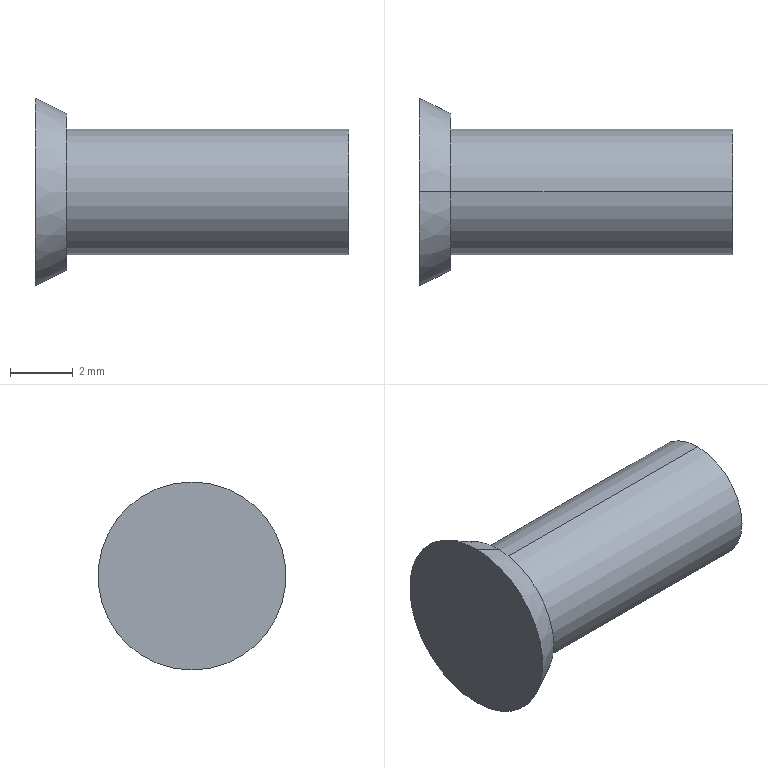Part | SolidWorks | features Revolution 1 | 1 solid | 7 faces | box 10 x 6 x 6 mm | volume 136.921 mm3 | plane 3 | cylinder 2 | cone 2 | commonest cylinder face diameters 4 x2
STEP:
#1=CARTESIAN_POINT('',(1.,0.,-2.));
#2=VERTEX_POINT('',#1);
#3=CARTESIAN_POINT('',(1.,0.,2.));
#4=VERTEX_POINT('',#3);
#5=CARTESIAN_POINT('',(1.,0.,0.));
#6=DIRECTION('',(1.,0.,0.));
#7=DIRECTION('',(0.,0.,-1.));
#8=AXIS2_PLACEMENT_3D('',#5,#6,#7);
#9=CIRCLE('',#8,2.);
#10=EDGE_CURVE('',#2,#4,#9,.T.);
#11=ORIENTED_EDGE('',*,*,#10,.T.);
#12=CARTESIAN_POINT('',(10.,0.,2.));
#13=VERTEX_POINT('',#12);
#14=CARTESIAN_POINT('',(10.,0.,2.));
#15=DIRECTION('',(1.,0.,0.));
#16=VECTOR('',#15,1000.);
#17=LINE('',#14,#16);
#18=EDGE_CURVE('',#4,#13,#17,.T.);
#19=ORIENTED_EDGE('',*,*,#18,.T.);
#20=CARTESIAN_POINT('',(10.,0.,-2.));
#21=VERTEX_POINT('',#20);
#22=CARTESIAN_POINT('',(10.,0.,0.));
#23=DIRECTION('',(1.,0.,0.));
#24=DIRECTION('',(0.,0.,-1.));
#25=AXIS2_PLACEMENT_3D('',#22,#23,#24);
#26=CIRCLE('',#25,2.);
#27=EDGE_CURVE('',#21,#13,#26,.T.);
#28=ORIENTED_EDGE('',*,*,#27,.F.);
#29=CARTESIAN_POINT('',(10.,0.,-2.));
#30=DIRECTION('',(1.,0.,0.));
#31=VECTOR('',#30,1000.);
#32=LINE('',#29,#31);
#33=EDGE_CURVE('',#2,#21,#32,.T.);
#34=ORIENTED_EDGE('',*,*,#33,.F.);
#35=EDGE_LOOP('',(#11,#19,#28,#34));
#36=FACE_OUTER_BOUND('',#35,.T.);
#37=CARTESIAN_POINT('',(10.,0.,0.));
#38=DIRECTION('',(1.,0.,0.));
#39=DIRECTION('',(0.,0.,-1.));
#40=AXIS2_PLACEMENT_3D('',#37,#38,#39);
#41=CYLINDRICAL_SURFACE('',#40,2.);
#42=ADVANCED_FACE('',(#36),#41,.T.);
#43=CARTESIAN_POINT('',(1.,0.,-2.5));
#44=VERTEX_POINT('',#43);
#45=CARTESIAN_POINT('',(1.,0.,2.5));
#46=VERTEX_POINT('',#45);
#47=CARTESIAN_POINT('',(1.,0.,0.));
#48=DIRECTION('',(1.,0.,0.));
#49=DIRECTION('',(0.,0.,-1.));
#50=AXIS2_PLACEMENT_3D('',#47,#48,#49);
#51=CIRCLE('',#50,2.5);
#52=EDGE_CURVE('',#44,#46,#51,.T.);
#53=ORIENTED_EDGE('',*,*,#52,.F.);
#54=CARTESIAN_POINT('',(0.,0.,-3.));
#55=VERTEX_POINT('',#54);
#56=CARTESIAN_POINT('',(1.,0.,-2.5));
#57=DIRECTION('',(-0.8944,0.,-0.4472));
#58=VECTOR('',#57,1000.);
#59=LINE('',#56,#58);
#60=EDGE_CURVE('',#44,#55,#59,.T.);
#61=ORIENTED_EDGE('',*,*,#60,.T.);
#62=CARTESIAN_POINT('',(0.,0.,3.));
#63=VERTEX_POINT('',#62);
#64=CARTESIAN_POINT('',(0.,0.,0.));
#65=DIRECTION('',(1.,0.,0.));
#66=DIRECTION('',(0.,0.,-1.));
#67=AXIS2_PLACEMENT_3D('',#64,#65,#66);
#68=CIRCLE('',#67,3.);
#69=EDGE_CURVE('',#55,#63,#68,.T.);
#70=ORIENTED_EDGE('',*,*,#69,.T.);
#71=CARTESIAN_POINT('',(1.,0.,2.5));
#72=DIRECTION('',(-0.8944,0.,0.4472));
#73=VECTOR('',#72,1000.);
#74=LINE('',#71,#73);
#75=EDGE_CURVE('',#46,#63,#74,.T.);
#76=ORIENTED_EDGE('',*,*,#75,.F.);
#77=EDGE_LOOP('',(#53,#61,#70,#76));
#78=FACE_OUTER_BOUND('',#77,.T.);
#79=CARTESIAN_POINT('',(1.,0.,0.));
#80=DIRECTION('',(-1.,0.,0.));
#81=DIRECTION('',(0.,0.,1.));
#82=AXIS2_PLACEMENT_3D('',#79,#80,#81);
#83=CONICAL_SURFACE('',#82,2.5,0.4636);
#84=ADVANCED_FACE('',(#78),#83,.T.);
#85=CARTESIAN_POINT('',(0.,0.,0.));
#86=DIRECTION('',(1.,0.,0.));
#87=DIRECTION('',(0.,0.,-1.));
#88=AXIS2_PLACEMENT_3D('',#85,#86,#87);
#89=CIRCLE('',#88,3.);
#90=EDGE_CURVE('',#63,#55,#89,.T.);
#91=ORIENTED_EDGE('',*,*,#90,.F.);
#92=ORIENTED_EDGE('',*,*,#69,.F.);
#93=EDGE_LOOP('',(#91,#92));
#94=FACE_OUTER_BOUND('',#93,.T.);
#95=CARTESIAN_POINT('',(0.,0.,0.));
#96=DIRECTION('',(-1.,0.,0.));
#97=DIRECTION('',(0.,0.,1.));
#98=AXIS2_PLACEMENT_3D('',#95,#96,#97);
#99=PLANE('',#98);
#100=ADVANCED_FACE('',(#94),#99,.T.);
#101=ORIENTED_EDGE('',*,*,#60,.F.);
#102=CARTESIAN_POINT('',(1.,0.,0.));
#103=DIRECTION('',(1.,0.,0.));
#104=DIRECTION('',(0.,0.,-1.));
#105=AXIS2_PLACEMENT_3D('',#102,#103,#104);
#106=CIRCLE('',#105,2.5);
#107=EDGE_CURVE('',#46,#44,#106,.T.);
#108=ORIENTED_EDGE('',*,*,#107,.F.);
#109=ORIENTED_EDGE('',*,*,#75,.T.);
#110=ORIENTED_EDGE('',*,*,#90,.T.);
#111=EDGE_LOOP('',(#101,#108,#109,#110));
#112=FACE_OUTER_BOUND('',#111,.T.);
#113=CARTESIAN_POINT('',(1.,0.,0.));
#114=DIRECTION('',(-1.,0.,0.));
#115=DIRECTION('',(0.,0.,1.));
#116=AXIS2_PLACEMENT_3D('',#113,#114,#115);
#117=CONICAL_SURFACE('',#116,2.5,0.4636);
#118=ADVANCED_FACE('',(#112),#117,.T.);
#119=ORIENTED_EDGE('',*,*,#107,.T.);
#120=ORIENTED_EDGE('',*,*,#52,.T.);
#121=EDGE_LOOP('',(#119,#120));
#122=FACE_OUTER_BOUND('',#121,.T.);
#123=ORIENTED_EDGE('',*,*,#10,.F.);
#124=CARTESIAN_POINT('',(1.,0.,0.));
#125=DIRECTION('',(1.,0.,0.));
#126=DIRECTION('',(0.,0.,-1.));
#127=AXIS2_PLACEMENT_3D('',#124,#125,#126);
#128=CIRCLE('',#127,2.);
#129=EDGE_CURVE('',#4,#2,#128,.T.);
#130=ORIENTED_EDGE('',*,*,#129,.F.);
#131=EDGE_LOOP('',(#123,#130));
#132=FACE_BOUND('',#131,.T.);
#133=CARTESIAN_POINT('',(1.,2.5,0.));
#134=DIRECTION('',(1.,0.,0.));
#135=DIRECTION('',(0.,0.,-1.));
#136=AXIS2_PLACEMENT_3D('',#133,#134,#135);
#137=PLANE('',#136);
#138=ADVANCED_FACE('',(#122,#132),#137,.T.);
#139=ORIENTED_EDGE('',*,*,#18,.F.);
#140=ORIENTED_EDGE('',*,*,#129,.T.);
#141=ORIENTED_EDGE('',*,*,#33,.T.);
#142=CARTESIAN_POINT('',(10.,0.,0.));
#143=DIRECTION('',(1.,0.,0.));
#144=DIRECTION('',(0.,0.,-1.));
#145=AXIS2_PLACEMENT_3D('',#142,#143,#144);
#146=CIRCLE('',#145,2.);
#147=EDGE_CURVE('',#13,#21,#146,.T.);
#148=ORIENTED_EDGE('',*,*,#147,.F.);
#149=EDGE_LOOP('',(#139,#140,#141,#148));
#150=FACE_OUTER_BOUND('',#149,.T.);
#151=CARTESIAN_POINT('',(10.,0.,0.));
#152=DIRECTION('',(1.,0.,0.));
#153=DIRECTION('',(0.,0.,-1.));
#154=AXIS2_PLACEMENT_3D('',#151,#152,#153);
#155=CYLINDRICAL_SURFACE('',#154,2.);
#156=ADVANCED_FACE('',(#150),#155,.T.);
#157=ORIENTED_EDGE('',*,*,#27,.T.);
#158=ORIENTED_EDGE('',*,*,#147,.T.);
#159=EDGE_LOOP('',(#157,#158));
#160=FACE_OUTER_BOUND('',#159,.T.);
#161=CARTESIAN_POINT('',(10.,2.,0.));
#162=DIRECTION('',(1.,0.,0.));
#163=DIRECTION('',(0.,0.,-1.));
#164=AXIS2_PLACEMENT_3D('',#161,#162,#163);
#165=PLANE('',#164);
#166=ADVANCED_FACE('',(#160),#165,.T.);
#167=CLOSED_SHELL('',(#42,#84,#100,#118,#138,#156,#166));
#168=MANIFOLD_SOLID_BREP('',#167);
#169=CARTESIAN_POINT('',(0.,0.,0.));
#170=DIRECTION('',(0.,0.,1.));
#171=DIRECTION('',(1.,0.,0.));
#172=AXIS2_PLACEMENT_3D('',#169,#170,#171);
#173=(LENGTH_UNIT()NAMED_UNIT(*)SI_UNIT(.MILLI.,.METRE.));
#174=UNCERTAINTY_MEASURE_WITH_UNIT(LENGTH_MEASURE(0.00001),#173,'','');
#175=(NAMED_UNIT(*)PLANE_ANGLE_UNIT()SI_UNIT($,.RADIAN.));
#176=(NAMED_UNIT(*)SI_UNIT($,.STERADIAN.)SOLID_ANGLE_UNIT());
#177=(GEOMETRIC_REPRESENTATION_CONTEXT(3)GLOBAL_UNCERTAINTY_ASSIGNED_CONTEXT((#174))GLOBAL_UNIT_ASSIGNED_CONTEXT((#173,#175,#176))REPRESENTATION_CONTEXT('',''));
#178=ADVANCED_BREP_SHAPE_REPRESENTATION('',(#168,#172),#177);